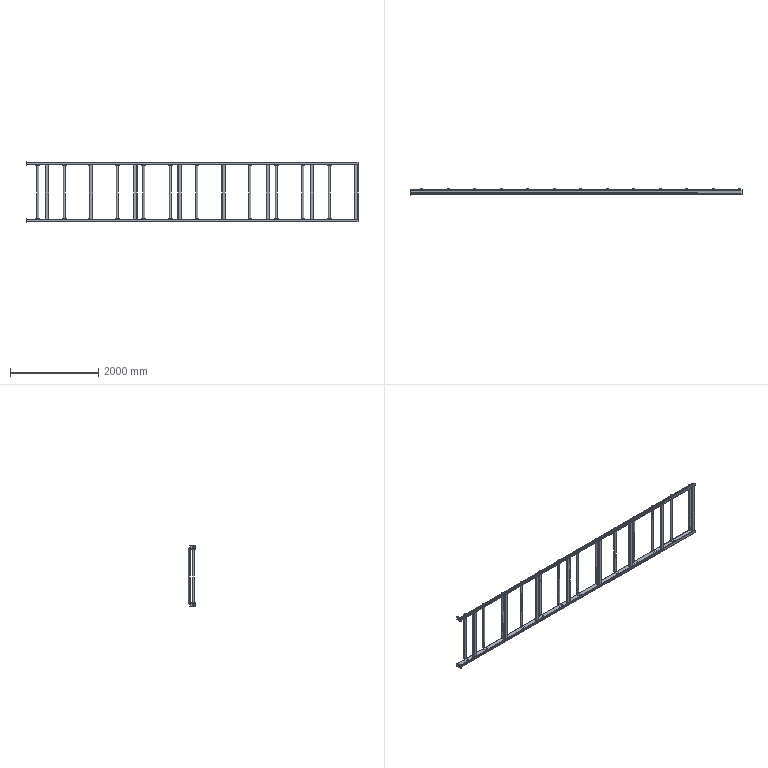Part | SolidWorks | features ReferencePattern 36, LocalLPattern 1 | 55 solids | 1986 faces | box 7516 x 170 x 1380 mm | volume 38650650 mm3 | cylinder 1066 | cone 468 | plane 452 | commonest cylinder face diameters 5.5 x352 5.61 x176 6.6 x176 15 x78 16 x52 17 x52